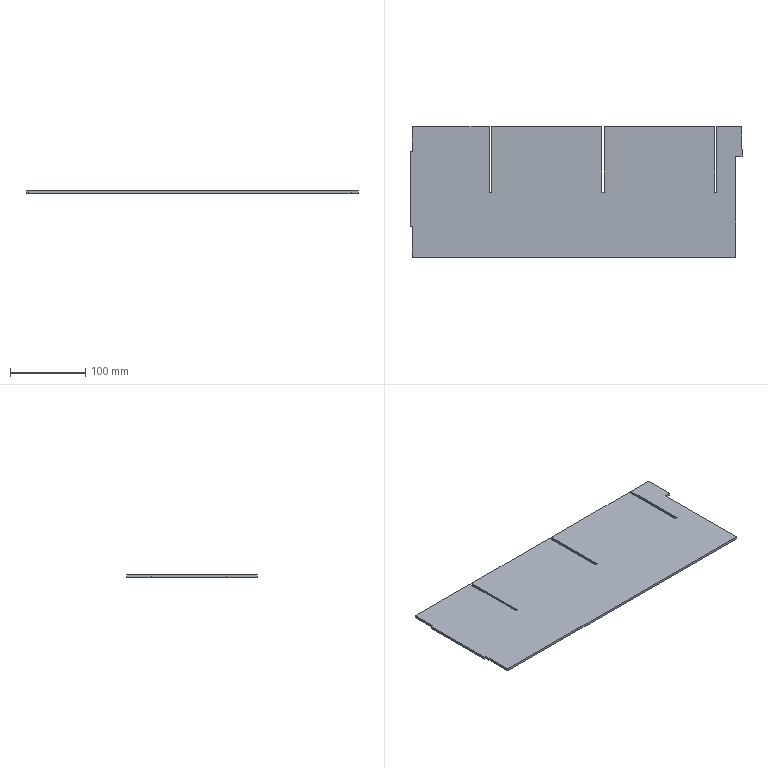Part | SolidWorks | features FlatPattern 1, SMBaseFlange 1, SheetMetal 1 | 1 solid | 24 faces | box 442 x 173.7 x 3.2 mm | volume 238742 mm3 | plane 24
STEP:
#1=CARTESIAN_POINT('',(-658.5,-13.627,0.));
#2=VERTEX_POINT('',#1);
#3=CARTESIAN_POINT('',(-658.5,-46.127,0.));
#4=VERTEX_POINT('',#3);
#5=CARTESIAN_POINT('',(-658.5,-13.627,0.));
#6=DIRECTION('',(0.,-1.,0.));
#7=VECTOR('',#6,1000.);
#8=LINE('',#5,#7);
#9=EDGE_CURVE('',#2,#4,#8,.T.);
#10=ORIENTED_EDGE('',*,*,#9,.T.);
#11=CARTESIAN_POINT('',(-658.5,-46.127,3.2));
#12=VERTEX_POINT('',#11);
#13=CARTESIAN_POINT('',(-658.5,-46.127,3.2));
#14=DIRECTION('',(0.,0.,-1.));
#15=VECTOR('',#14,1000.);
#16=LINE('',#13,#15);
#17=EDGE_CURVE('',#12,#4,#16,.T.);
#18=ORIENTED_EDGE('',*,*,#17,.F.);
#19=CARTESIAN_POINT('',(-658.5,-13.627,3.2));
#20=VERTEX_POINT('',#19);
#21=CARTESIAN_POINT('',(-658.5,-13.627,3.2));
#22=DIRECTION('',(0.,-1.,0.));
#23=VECTOR('',#22,1000.);
#24=LINE('',#21,#23);
#25=EDGE_CURVE('',#20,#12,#24,.T.);
#26=ORIENTED_EDGE('',*,*,#25,.F.);
#27=CARTESIAN_POINT('',(-658.5,-13.627,3.2));
#28=DIRECTION('',(0.,0.,-1.));
#29=VECTOR('',#28,1000.);
#30=LINE('',#27,#29);
#31=EDGE_CURVE('',#20,#2,#30,.T.);
#32=ORIENTED_EDGE('',*,*,#31,.T.);
#33=EDGE_LOOP('',(#10,#18,#26,#32));
#34=FACE_OUTER_BOUND('',#33,.T.);
#35=CARTESIAN_POINT('',(-658.5,-13.627,3.2));
#36=DIRECTION('',(1.,0.,0.));
#37=DIRECTION('',(0.,1.,0.));
#38=AXIS2_PLACEMENT_3D('',#35,#36,#37);
#39=PLANE('',#38);
#40=ADVANCED_FACE('',(#34),#39,.F.);
#41=CARTESIAN_POINT('',(-661.5,-46.127,0.));
#42=VERTEX_POINT('',#41);
#43=CARTESIAN_POINT('',(-658.5,-46.127,0.));
#44=DIRECTION('',(-1.,0.,0.));
#45=VECTOR('',#44,1000.);
#46=LINE('',#43,#45);
#47=EDGE_CURVE('',#4,#42,#46,.T.);
#48=ORIENTED_EDGE('',*,*,#47,.T.);
#49=CARTESIAN_POINT('',(-661.5,-46.127,3.2));
#50=VERTEX_POINT('',#49);
#51=CARTESIAN_POINT('',(-661.5,-46.127,3.2));
#52=DIRECTION('',(0.,0.,-1.));
#53=VECTOR('',#52,1000.);
#54=LINE('',#51,#53);
#55=EDGE_CURVE('',#50,#42,#54,.T.);
#56=ORIENTED_EDGE('',*,*,#55,.F.);
#57=CARTESIAN_POINT('',(-658.5,-46.127,3.2));
#58=DIRECTION('',(-1.,0.,0.));
#59=VECTOR('',#58,1000.);
#60=LINE('',#57,#59);
#61=EDGE_CURVE('',#12,#50,#60,.T.);
#62=ORIENTED_EDGE('',*,*,#61,.F.);
#63=ORIENTED_EDGE('',*,*,#17,.T.);
#64=EDGE_LOOP('',(#48,#56,#62,#63));
#65=FACE_OUTER_BOUND('',#64,.T.);
#66=CARTESIAN_POINT('',(-658.5,-46.127,3.2));
#67=DIRECTION('',(0.,-1.,0.));
#68=DIRECTION('',(1.,0.,0.));
#69=AXIS2_PLACEMENT_3D('',#66,#67,#68);
#70=PLANE('',#69);
#71=ADVANCED_FACE('',(#65),#70,.F.);
#72=CARTESIAN_POINT('',(-661.5,-146.127,0.));
#73=VERTEX_POINT('',#72);
#74=CARTESIAN_POINT('',(-661.5,-46.127,0.));
#75=DIRECTION('',(0.,-1.,0.));
#76=VECTOR('',#75,1000.);
#77=LINE('',#74,#76);
#78=EDGE_CURVE('',#42,#73,#77,.T.);
#79=ORIENTED_EDGE('',*,*,#78,.T.);
#80=CARTESIAN_POINT('',(-661.5,-146.127,3.2));
#81=VERTEX_POINT('',#80);
#82=CARTESIAN_POINT('',(-661.5,-146.127,3.2));
#83=DIRECTION('',(0.,0.,-1.));
#84=VECTOR('',#83,1000.);
#85=LINE('',#82,#84);
#86=EDGE_CURVE('',#81,#73,#85,.T.);
#87=ORIENTED_EDGE('',*,*,#86,.F.);
#88=CARTESIAN_POINT('',(-661.5,-46.127,3.2));
#89=DIRECTION('',(0.,-1.,0.));
#90=VECTOR('',#89,1000.);
#91=LINE('',#88,#90);
#92=EDGE_CURVE('',#50,#81,#91,.T.);
#93=ORIENTED_EDGE('',*,*,#92,.F.);
#94=ORIENTED_EDGE('',*,*,#55,.T.);
#95=EDGE_LOOP('',(#79,#87,#93,#94));
#96=FACE_OUTER_BOUND('',#95,.T.);
#97=CARTESIAN_POINT('',(-661.5,-46.127,3.2));
#98=DIRECTION('',(1.,0.,0.));
#99=DIRECTION('',(0.,1.,0.));
#100=AXIS2_PLACEMENT_3D('',#97,#98,#99);
#101=PLANE('',#100);
#102=ADVANCED_FACE('',(#96),#101,.F.);
#103=CARTESIAN_POINT('',(-658.5,-146.127,0.));
#104=VERTEX_POINT('',#103);
#105=CARTESIAN_POINT('',(-658.5,-146.127,0.));
#106=DIRECTION('',(1.,0.,0.));
#107=VECTOR('',#106,1000.);
#108=LINE('',#105,#107);
#109=EDGE_CURVE('',#73,#104,#108,.T.);
#110=ORIENTED_EDGE('',*,*,#109,.T.);
#111=CARTESIAN_POINT('',(-658.5,-146.127,3.2));
#112=VERTEX_POINT('',#111);
#113=CARTESIAN_POINT('',(-658.5,-146.127,3.2));
#114=DIRECTION('',(0.,0.,-1.));
#115=VECTOR('',#114,1000.);
#116=LINE('',#113,#115);
#117=EDGE_CURVE('',#112,#104,#116,.T.);
#118=ORIENTED_EDGE('',*,*,#117,.F.);
#119=CARTESIAN_POINT('',(-658.5,-146.127,3.2));
#120=DIRECTION('',(1.,0.,0.));
#121=VECTOR('',#120,1000.);
#122=LINE('',#119,#121);
#123=EDGE_CURVE('',#81,#112,#122,.T.);
#124=ORIENTED_EDGE('',*,*,#123,.F.);
#125=ORIENTED_EDGE('',*,*,#86,.T.);
#126=EDGE_LOOP('',(#110,#118,#124,#125));
#127=FACE_OUTER_BOUND('',#126,.T.);
#128=CARTESIAN_POINT('',(-658.5,-146.127,3.2));
#129=DIRECTION('',(0.,1.,0.));
#130=DIRECTION('',(0.,0.,1.));
#131=AXIS2_PLACEMENT_3D('',#128,#129,#130);
#132=PLANE('',#131);
#133=ADVANCED_FACE('',(#127),#132,.F.);
#134=CARTESIAN_POINT('',(-658.5,-187.327,0.));
#135=VERTEX_POINT('',#134);
#136=CARTESIAN_POINT('',(-658.5,-146.127,0.));
#137=DIRECTION('',(0.,-1.,0.));
#138=VECTOR('',#137,1000.);
#139=LINE('',#136,#138);
#140=EDGE_CURVE('',#104,#135,#139,.T.);
#141=ORIENTED_EDGE('',*,*,#140,.T.);
#142=CARTESIAN_POINT('',(-658.5,-187.327,3.2));
#143=VERTEX_POINT('',#142);
#144=CARTESIAN_POINT('',(-658.5,-187.327,3.2));
#145=DIRECTION('',(0.,0.,-1.));
#146=VECTOR('',#145,1000.);
#147=LINE('',#144,#146);
#148=EDGE_CURVE('',#143,#135,#147,.T.);
#149=ORIENTED_EDGE('',*,*,#148,.F.);
#150=CARTESIAN_POINT('',(-658.5,-146.127,3.2));
#151=DIRECTION('',(0.,-1.,0.));
#152=VECTOR('',#151,1000.);
#153=LINE('',#150,#152);
#154=EDGE_CURVE('',#112,#143,#153,.T.);
#155=ORIENTED_EDGE('',*,*,#154,.F.);
#156=ORIENTED_EDGE('',*,*,#117,.T.);
#157=EDGE_LOOP('',(#141,#149,#155,#156));
#158=FACE_OUTER_BOUND('',#157,.T.);
#159=CARTESIAN_POINT('',(-658.5,-146.127,3.2));
#160=DIRECTION('',(1.,0.,0.));
#161=DIRECTION('',(0.,1.,0.));
#162=AXIS2_PLACEMENT_3D('',#159,#160,#161);
#163=PLANE('',#162);
#164=ADVANCED_FACE('',(#158),#163,.F.);
#165=CARTESIAN_POINT('',(-227.8,-187.327,0.));
#166=VERTEX_POINT('',#165);
#167=CARTESIAN_POINT('',(-227.8,-187.327,0.));
#168=DIRECTION('',(1.,0.,0.));
#169=VECTOR('',#168,1000.);
#170=LINE('',#167,#169);
#171=EDGE_CURVE('',#135,#166,#170,.T.);
#172=ORIENTED_EDGE('',*,*,#171,.T.);
#173=CARTESIAN_POINT('',(-227.8,-187.327,3.2));
#174=VERTEX_POINT('',#173);
#175=CARTESIAN_POINT('',(-227.8,-187.327,3.2));
#176=DIRECTION('',(0.,0.,-1.));
#177=VECTOR('',#176,1000.);
#178=LINE('',#175,#177);
#179=EDGE_CURVE('',#174,#166,#178,.T.);
#180=ORIENTED_EDGE('',*,*,#179,.F.);
#181=CARTESIAN_POINT('',(-227.8,-187.327,3.2));
#182=DIRECTION('',(1.,0.,0.));
#183=VECTOR('',#182,1000.);
#184=LINE('',#181,#183);
#185=EDGE_CURVE('',#143,#174,#184,.T.);
#186=ORIENTED_EDGE('',*,*,#185,.F.);
#187=ORIENTED_EDGE('',*,*,#148,.T.);
#188=EDGE_LOOP('',(#172,#180,#186,#187));
#189=FACE_OUTER_BOUND('',#188,.T.);
#190=CARTESIAN_POINT('',(-227.8,-187.327,3.2));
#191=DIRECTION('',(0.,1.,0.));
#192=DIRECTION('',(-1.,0.,0.));
#193=AXIS2_PLACEMENT_3D('',#190,#191,#192);
#194=PLANE('',#193);
#195=ADVANCED_FACE('',(#189),#194,.F.);
#196=CARTESIAN_POINT('',(-227.8,-53.327,0.));
#197=VERTEX_POINT('',#196);
#198=CARTESIAN_POINT('',(-227.8,-53.327,0.));
#199=DIRECTION('',(0.,1.,0.));
#200=VECTOR('',#199,1000.);
#201=LINE('',#198,#200);
#202=EDGE_CURVE('',#166,#197,#201,.T.);
#203=ORIENTED_EDGE('',*,*,#202,.T.);
#204=CARTESIAN_POINT('',(-227.8,-53.327,3.2));
#205=VERTEX_POINT('',#204);
#206=CARTESIAN_POINT('',(-227.8,-53.327,3.2));
#207=DIRECTION('',(0.,0.,-1.));
#208=VECTOR('',#207,1000.);
#209=LINE('',#206,#208);
#210=EDGE_CURVE('',#205,#197,#209,.T.);
#211=ORIENTED_EDGE('',*,*,#210,.F.);
#212=CARTESIAN_POINT('',(-227.8,-53.327,3.2));
#213=DIRECTION('',(0.,1.,0.));
#214=VECTOR('',#213,1000.);
#215=LINE('',#212,#214);
#216=EDGE_CURVE('',#174,#205,#215,.T.);
#217=ORIENTED_EDGE('',*,*,#216,.F.);
#218=ORIENTED_EDGE('',*,*,#179,.T.);
#219=EDGE_LOOP('',(#203,#211,#217,#218));
#220=FACE_OUTER_BOUND('',#219,.T.);
#221=CARTESIAN_POINT('',(-227.8,-53.327,3.2));
#222=DIRECTION('',(-1.,0.,0.));
#223=DIRECTION('',(0.,-1.,0.));
#224=AXIS2_PLACEMENT_3D('',#221,#222,#223);
#225=PLANE('',#224);
#226=ADVANCED_FACE('',(#220),#225,.F.);
#227=CARTESIAN_POINT('',(-219.5,-53.327,0.));
#228=VERTEX_POINT('',#227);
#229=CARTESIAN_POINT('',(-227.8,-53.327,0.));
#230=DIRECTION('',(1.,0.,0.));
#231=VECTOR('',#230,1000.);
#232=LINE('',#229,#231);
#233=EDGE_CURVE('',#197,#228,#232,.T.);
#234=ORIENTED_EDGE('',*,*,#233,.T.);
#235=CARTESIAN_POINT('',(-219.5,-53.327,3.2));
#236=VERTEX_POINT('',#235);
#237=CARTESIAN_POINT('',(-219.5,-53.327,3.2));
#238=DIRECTION('',(0.,0.,-1.));
#239=VECTOR('',#238,1000.);
#240=LINE('',#237,#239);
#241=EDGE_CURVE('',#236,#228,#240,.T.);
#242=ORIENTED_EDGE('',*,*,#241,.F.);
#243=CARTESIAN_POINT('',(-227.8,-53.327,3.2));
#244=DIRECTION('',(1.,0.,0.));
#245=VECTOR('',#244,1000.);
#246=LINE('',#243,#245);
#247=EDGE_CURVE('',#205,#236,#246,.T.);
#248=ORIENTED_EDGE('',*,*,#247,.F.);
#249=ORIENTED_EDGE('',*,*,#210,.T.);
#250=EDGE_LOOP('',(#234,#242,#248,#249));
#251=FACE_OUTER_BOUND('',#250,.T.);
#252=CARTESIAN_POINT('',(-227.8,-53.327,3.2));
#253=DIRECTION('',(0.,1.,0.));
#254=DIRECTION('',(-1.,0.,0.));
#255=AXIS2_PLACEMENT_3D('',#252,#253,#254);
#256=PLANE('',#255);
#257=ADVANCED_FACE('',(#251),#256,.F.);
#258=CARTESIAN_POINT('',(-219.5,-13.627,0.));
#259=VERTEX_POINT('',#258);
#260=CARTESIAN_POINT('',(-219.5,-53.327,0.));
#261=DIRECTION('',(0.,1.,0.));
#262=VECTOR('',#261,1000.);
#263=LINE('',#260,#262);
#264=EDGE_CURVE('',#228,#259,#263,.T.);
#265=ORIENTED_EDGE('',*,*,#264,.T.);
#266=CARTESIAN_POINT('',(-219.5,-13.627,3.2));
#267=VERTEX_POINT('',#266);
#268=CARTESIAN_POINT('',(-219.5,-13.627,3.2));
#269=DIRECTION('',(0.,0.,-1.));
#270=VECTOR('',#269,1000.);
#271=LINE('',#268,#270);
#272=EDGE_CURVE('',#267,#259,#271,.T.);
#273=ORIENTED_EDGE('',*,*,#272,.F.);
#274=CARTESIAN_POINT('',(-219.5,-53.327,3.2));
#275=DIRECTION('',(0.,1.,0.));
#276=VECTOR('',#275,1000.);
#277=LINE('',#274,#276);
#278=EDGE_CURVE('',#236,#267,#277,.T.);
#279=ORIENTED_EDGE('',*,*,#278,.F.);
#280=ORIENTED_EDGE('',*,*,#241,.T.);
#281=EDGE_LOOP('',(#265,#273,#279,#280));
#282=FACE_OUTER_BOUND('',#281,.T.);
#283=CARTESIAN_POINT('',(-219.5,-53.327,3.2));
#284=DIRECTION('',(-1.,0.,0.));
#285=DIRECTION('',(0.,-1.,0.));
#286=AXIS2_PLACEMENT_3D('',#283,#284,#285);
#287=PLANE('',#286);
#288=ADVANCED_FACE('',(#282),#287,.F.);
#289=CARTESIAN_POINT('',(-252.8,-13.627,0.));
#290=VERTEX_POINT('',#289);
#291=CARTESIAN_POINT('',(-219.5,-13.627,0.));
#292=DIRECTION('',(-1.,0.,0.));
#293=VECTOR('',#292,1000.);
#294=LINE('',#291,#293);
#295=EDGE_CURVE('',#259,#290,#294,.T.);
#296=ORIENTED_EDGE('',*,*,#295,.T.);
#297=CARTESIAN_POINT('',(-252.8,-13.627,3.2));
#298=VERTEX_POINT('',#297);
#299=CARTESIAN_POINT('',(-252.8,-13.627,3.2));
#300=DIRECTION('',(0.,0.,-1.));
#301=VECTOR('',#300,1000.);
#302=LINE('',#299,#301);
#303=EDGE_CURVE('',#298,#290,#302,.T.);
#304=ORIENTED_EDGE('',*,*,#303,.F.);
#305=CARTESIAN_POINT('',(-219.5,-13.627,3.2));
#306=DIRECTION('',(-1.,0.,0.));
#307=VECTOR('',#306,1000.);
#308=LINE('',#305,#307);
#309=EDGE_CURVE('',#267,#298,#308,.T.);
#310=ORIENTED_EDGE('',*,*,#309,.F.);
#311=ORIENTED_EDGE('',*,*,#272,.T.);
#312=EDGE_LOOP('',(#296,#304,#310,#311));
#313=FACE_OUTER_BOUND('',#312,.T.);
#314=CARTESIAN_POINT('',(-219.5,-13.627,3.2));
#315=DIRECTION('',(0.,-1.,0.));
#316=DIRECTION('',(1.,0.,0.));
#317=AXIS2_PLACEMENT_3D('',#314,#315,#316);
#318=PLANE('',#317);
#319=ADVANCED_FACE('',(#313),#318,.F.);
#320=CARTESIAN_POINT('',(-252.8,-100.627,0.));
#321=VERTEX_POINT('',#320);
#322=CARTESIAN_POINT('',(-252.8,-13.627,0.));
#323=DIRECTION('',(0.,-1.,0.));
#324=VECTOR('',#323,1000.);
#325=LINE('',#322,#324);
#326=EDGE_CURVE('',#290,#321,#325,.T.);
#327=ORIENTED_EDGE('',*,*,#326,.T.);
#328=CARTESIAN_POINT('',(-252.8,-100.627,3.2));
#329=VERTEX_POINT('',#328);
#330=CARTESIAN_POINT('',(-252.8,-100.627,3.2));
#331=DIRECTION('',(0.,0.,-1.));
#332=VECTOR('',#331,1000.);
#333=LINE('',#330,#332);
#334=EDGE_CURVE('',#329,#321,#333,.T.);
#335=ORIENTED_EDGE('',*,*,#334,.F.);
#336=CARTESIAN_POINT('',(-252.8,-13.627,3.2));
#337=DIRECTION('',(0.,-1.,0.));
#338=VECTOR('',#337,1000.);
#339=LINE('',#336,#338);
#340=EDGE_CURVE('',#298,#329,#339,.T.);
#341=ORIENTED_EDGE('',*,*,#340,.F.);
#342=ORIENTED_EDGE('',*,*,#303,.T.);
#343=EDGE_LOOP('',(#327,#335,#341,#342));
#344=FACE_OUTER_BOUND('',#343,.T.);
#345=CARTESIAN_POINT('',(-252.8,-13.627,3.2));
#346=DIRECTION('',(1.,0.,0.));
#347=DIRECTION('',(0.,0.,-1.));
#348=AXIS2_PLACEMENT_3D('',#345,#346,#347);
#349=PLANE('',#348);
#350=ADVANCED_FACE('',(#344),#349,.F.);
#351=CARTESIAN_POINT('',(-256.,-100.627,0.));
#352=VERTEX_POINT('',#351);
#353=CARTESIAN_POINT('',(-252.8,-100.627,0.));
#354=DIRECTION('',(-1.,0.,0.));
#355=VECTOR('',#354,1000.);
#356=LINE('',#353,#355);
#357=EDGE_CURVE('',#321,#352,#356,.T.);
#358=ORIENTED_EDGE('',*,*,#357,.T.);
#359=CARTESIAN_POINT('',(-256.,-100.627,3.2));
#360=VERTEX_POINT('',#359);
#361=CARTESIAN_POINT('',(-256.,-100.627,3.2));
#362=DIRECTION('',(0.,0.,-1.));
#363=VECTOR('',#362,1000.);
#364=LINE('',#361,#363);
#365=EDGE_CURVE('',#360,#352,#364,.T.);
#366=ORIENTED_EDGE('',*,*,#365,.F.);
#367=CARTESIAN_POINT('',(-252.8,-100.627,3.2));
#368=DIRECTION('',(-1.,0.,0.));
#369=VECTOR('',#368,1000.);
#370=LINE('',#367,#369);
#371=EDGE_CURVE('',#329,#360,#370,.T.);
#372=ORIENTED_EDGE('',*,*,#371,.F.);
#373=ORIENTED_EDGE('',*,*,#334,.T.);
#374=EDGE_LOOP('',(#358,#366,#372,#373));
#375=FACE_OUTER_BOUND('',#374,.T.);
#376=CARTESIAN_POINT('',(-252.8,-100.627,3.2));
#377=DIRECTION('',(0.,-1.,0.));
#378=DIRECTION('',(0.,0.,-1.));
#379=AXIS2_PLACEMENT_3D('',#376,#377,#378);
#380=PLANE('',#379);
#381=ADVANCED_FACE('',(#375),#380,.F.);
#382=CARTESIAN_POINT('',(-256.,-13.627,0.));
#383=VERTEX_POINT('',#382);
#384=CARTESIAN_POINT('',(-256.,-100.627,0.));
#385=DIRECTION('',(0.,1.,0.));
#386=VECTOR('',#385,1000.);
#387=LINE('',#384,#386);
#388=EDGE_CURVE('',#352,#383,#387,.T.);
#389=ORIENTED_EDGE('',*,*,#388,.T.);
#390=CARTESIAN_POINT('',(-256.,-13.627,3.2));
#391=VERTEX_POINT('',#390);
#392=CARTESIAN_POINT('',(-256.,-13.627,3.2));
#393=DIRECTION('',(0.,0.,-1.));
#394=VECTOR('',#393,1000.);
#395=LINE('',#392,#394);
#396=EDGE_CURVE('',#391,#383,#395,.T.);
#397=ORIENTED_EDGE('',*,*,#396,.F.);
#398=CARTESIAN_POINT('',(-256.,-100.627,3.2));
#399=DIRECTION('',(0.,1.,0.));
#400=VECTOR('',#399,1000.);
#401=LINE('',#398,#400);
#402=EDGE_CURVE('',#360,#391,#401,.T.);
#403=ORIENTED_EDGE('',*,*,#402,.F.);
#404=ORIENTED_EDGE('',*,*,#365,.T.);
#405=EDGE_LOOP('',(#389,#397,#403,#404));
#406=FACE_OUTER_BOUND('',#405,.T.);
#407=CARTESIAN_POINT('',(-256.,-100.627,3.2));
#408=DIRECTION('',(-1.,0.,0.));
#409=DIRECTION('',(0.,0.,1.));
#410=AXIS2_PLACEMENT_3D('',#407,#408,#409);
#411=PLANE('',#410);
#412=ADVANCED_FACE('',(#406),#411,.F.);
#413=CARTESIAN_POINT('',(-402.8,-13.627,0.));
#414=VERTEX_POINT('',#413);
#415=CARTESIAN_POINT('',(-256.,-13.627,0.));
#416=DIRECTION('',(-1.,0.,0.));
#417=VECTOR('',#416,1000.);
#418=LINE('',#415,#417);
#419=EDGE_CURVE('',#383,#414,#418,.T.);
#420=ORIENTED_EDGE('',*,*,#419,.T.);
#421=CARTESIAN_POINT('',(-402.8,-13.627,3.2));
#422=VERTEX_POINT('',#421);
#423=CARTESIAN_POINT('',(-402.8,-13.627,3.2));
#424=DIRECTION('',(0.,0.,-1.));
#425=VECTOR('',#424,1000.);
#426=LINE('',#423,#425);
#427=EDGE_CURVE('',#422,#414,#426,.T.);
#428=ORIENTED_EDGE('',*,*,#427,.F.);
#429=CARTESIAN_POINT('',(-256.,-13.627,3.2));
#430=DIRECTION('',(-1.,0.,0.));
#431=VECTOR('',#430,1000.);
#432=LINE('',#429,#431);
#433=EDGE_CURVE('',#391,#422,#432,.T.);
#434=ORIENTED_EDGE('',*,*,#433,.F.);
#435=ORIENTED_EDGE('',*,*,#396,.T.);
#436=EDGE_LOOP('',(#420,#428,#434,#435));
#437=FACE_OUTER_BOUND('',#436,.T.);
#438=CARTESIAN_POINT('',(-256.,-13.627,3.2));
#439=DIRECTION('',(0.,-1.,0.));
#440=DIRECTION('',(1.,0.,0.));
#441=AXIS2_PLACEMENT_3D('',#438,#439,#440);
#442=PLANE('',#441);
#443=ADVANCED_FACE('',(#437),#442,.F.);
#444=CARTESIAN_POINT('',(-402.8,-100.627,0.));
#445=VERTEX_POINT('',#444);
#446=CARTESIAN_POINT('',(-402.8,-13.627,0.));
#447=DIRECTION('',(0.,-1.,0.));
#448=VECTOR('',#447,1000.);
#449=LINE('',#446,#448);
#450=EDGE_CURVE('',#414,#445,#449,.T.);
#451=ORIENTED_EDGE('',*,*,#450,.T.);
#452=CARTESIAN_POINT('',(-402.8,-100.627,3.2));
#453=VERTEX_POINT('',#452);
#454=CARTESIAN_POINT('',(-402.8,-100.627,3.2));
#455=DIRECTION('',(0.,0.,-1.));
#456=VECTOR('',#455,1000.);
#457=LINE('',#454,#456);
#458=EDGE_CURVE('',#453,#445,#457,.T.);
#459=ORIENTED_EDGE('',*,*,#458,.F.);
#460=CARTESIAN_POINT('',(-402.8,-13.627,3.2));
#461=DIRECTION('',(0.,-1.,0.));
#462=VECTOR('',#461,1000.);
#463=LINE('',#460,#462);
#464=EDGE_CURVE('',#422,#453,#463,.T.);
#465=ORIENTED_EDGE('',*,*,#464,.F.);
#466=ORIENTED_EDGE('',*,*,#427,.T.);
#467=EDGE_LOOP('',(#451,#459,#465,#466));
#468=FACE_OUTER_BOUND('',#467,.T.);
#469=CARTESIAN_POINT('',(-402.8,-13.627,3.2));
#470=DIRECTION('',(1.,0.,0.));
#471=DIRECTION('',(0.,1.,0.));
#472=AXIS2_PLACEMENT_3D('',#469,#470,#471);
#473=PLANE('',#472);
#474=ADVANCED_FACE('',(#468),#473,.F.);
#475=CARTESIAN_POINT('',(-406.,-100.627,0.));
#476=VERTEX_POINT('',#475);
#477=CARTESIAN_POINT('',(-402.8,-100.627,0.));
#478=DIRECTION('',(-1.,0.,0.));
#479=VECTOR('',#478,1000.);
#480=LINE('',#477,#479);
#481=EDGE_CURVE('',#445,#476,#480,.T.);
#482=ORIENTED_EDGE('',*,*,#481,.T.);
#483=CARTESIAN_POINT('',(-406.,-100.627,3.2));
#484=VERTEX_POINT('',#483);
#485=CARTESIAN_POINT('',(-406.,-100.627,3.2));
#486=DIRECTION('',(0.,0.,-1.));
#487=VECTOR('',#486,1000.);
#488=LINE('',#485,#487);
#489=EDGE_CURVE('',#484,#476,#488,.T.);
#490=ORIENTED_EDGE('',*,*,#489,.F.);
#491=CARTESIAN_POINT('',(-402.8,-100.627,3.2));
#492=DIRECTION('',(-1.,0.,0.));
#493=VECTOR('',#492,1000.);
#494=LINE('',#491,#493);
#495=EDGE_CURVE('',#453,#484,#494,.T.);
#496=ORIENTED_EDGE('',*,*,#495,.F.);
#497=ORIENTED_EDGE('',*,*,#458,.T.);
#498=EDGE_LOOP('',(#482,#490,#496,#497));
#499=FACE_OUTER_BOUND('',#498,.T.);
#500=CARTESIAN_POINT('',(-402.8,-100.627,3.2));
#501=DIRECTION('',(0.,-1.,0.));
#502=DIRECTION('',(0.,0.,-1.));
#503=AXIS2_PLACEMENT_3D('',#500,#501,#502);
#504=PLANE('',#503);
#505=ADVANCED_FACE('',(#499),#504,.F.);
#506=CARTESIAN_POINT('',(-406.,-13.627,0.));
#507=VERTEX_POINT('',#506);
#508=CARTESIAN_POINT('',(-406.,-100.627,0.));
#509=DIRECTION('',(0.,1.,0.));
#510=VECTOR('',#509,1000.);
#511=LINE('',#508,#510);
#512=EDGE_CURVE('',#476,#507,#511,.T.);
#513=ORIENTED_EDGE('',*,*,#512,.T.);
#514=CARTESIAN_POINT('',(-406.,-13.627,3.2));
#515=VERTEX_POINT('',#514);
#516=CARTESIAN_POINT('',(-406.,-13.627,3.2));
#517=DIRECTION('',(0.,0.,-1.));
#518=VECTOR('',#517,1000.);
#519=LINE('',#516,#518);
#520=EDGE_CURVE('',#515,#507,#519,.T.);
#521=ORIENTED_EDGE('',*,*,#520,.F.);
#522=CARTESIAN_POINT('',(-406.,-100.627,3.2));
#523=DIRECTION('',(0.,1.,0.));
#524=VECTOR('',#523,1000.);
#525=LINE('',#522,#524);
#526=EDGE_CURVE('',#484,#515,#525,.T.);
#527=ORIENTED_EDGE('',*,*,#526,.F.);
#528=ORIENTED_EDGE('',*,*,#489,.T.);
#529=EDGE_LOOP('',(#513,#521,#527,#528));
#530=FACE_OUTER_BOUND('',#529,.T.);
#531=CARTESIAN_POINT('',(-406.,-100.627,3.2));
#532=DIRECTION('',(-1.,0.,0.));
#533=DIRECTION('',(0.,-1.,0.));
#534=AXIS2_PLACEMENT_3D('',#531,#532,#533);
#535=PLANE('',#534);
#536=ADVANCED_FACE('',(#530),#535,.F.);
#537=CARTESIAN_POINT('',(-552.8,-13.627,0.));
#538=VERTEX_POINT('',#537);
#539=CARTESIAN_POINT('',(-406.,-13.627,0.));
#540=DIRECTION('',(-1.,0.,0.));
#541=VECTOR('',#540,1000.);
#542=LINE('',#539,#541);
#543=EDGE_CURVE('',#507,#538,#542,.T.);
#544=ORIENTED_EDGE('',*,*,#543,.T.);
#545=CARTESIAN_POINT('',(-552.8,-13.627,3.2));
#546=VERTEX_POINT('',#545);
#547=CARTESIAN_POINT('',(-552.8,-13.627,3.2));
#548=DIRECTION('',(0.,0.,-1.));
#549=VECTOR('',#548,1000.);
#550=LINE('',#547,#549);
#551=EDGE_CURVE('',#546,#538,#550,.T.);
#552=ORIENTED_EDGE('',*,*,#551,.F.);
#553=CARTESIAN_POINT('',(-406.,-13.627,3.2));
#554=DIRECTION('',(-1.,0.,0.));
#555=VECTOR('',#554,1000.);
#556=LINE('',#553,#555);
#557=EDGE_CURVE('',#515,#546,#556,.T.);
#558=ORIENTED_EDGE('',*,*,#557,.F.);
#559=ORIENTED_EDGE('',*,*,#520,.T.);
#560=EDGE_LOOP('',(#544,#552,#558,#559));
#561=FACE_OUTER_BOUND('',#560,.T.);
#562=CARTESIAN_POINT('',(-406.,-13.627,3.2));
#563=DIRECTION('',(0.,-1.,0.));
#564=DIRECTION('',(1.,0.,0.));
#565=AXIS2_PLACEMENT_3D('',#562,#563,#564);
#566=PLANE('',#565);
#567=ADVANCED_FACE('',(#561),#566,.F.);
#568=CARTESIAN_POINT('',(-552.8,-100.627,0.));
#569=VERTEX_POINT('',#568);
#570=CARTESIAN_POINT('',(-552.8,-13.627,0.));
#571=DIRECTION('',(0.,-1.,0.));
#572=VECTOR('',#571,1000.);
#573=LINE('',#570,#572);
#574=EDGE_CURVE('',#538,#569,#573,.T.);
#575=ORIENTED_EDGE('',*,*,#574,.T.);
#576=CARTESIAN_POINT('',(-552.8,-100.627,3.2));
#577=VERTEX_POINT('',#576);
#578=CARTESIAN_POINT('',(-552.8,-100.627,3.2));
#579=DIRECTION('',(0.,0.,-1.));
#580=VECTOR('',#579,1000.);
#581=LINE('',#578,#580);
#582=EDGE_CURVE('',#577,#569,#581,.T.);
#583=ORIENTED_EDGE('',*,*,#582,.F.);
#584=CARTESIAN_POINT('',(-552.8,-13.627,3.2));
#585=DIRECTION('',(0.,-1.,0.));
#586=VECTOR('',#585,1000.);
#587=LINE('',#584,#586);
#588=EDGE_CURVE('',#546,#577,#587,.T.);
#589=ORIENTED_EDGE('',*,*,#588,.F.);
#590=ORIENTED_EDGE('',*,*,#551,.T.);
#591=EDGE_LOOP('',(#575,#583,#589,#590));
#592=FACE_OUTER_BOUND('',#591,.T.);
#593=CARTESIAN_POINT('',(-552.8,-13.627,3.2));
#594=DIRECTION('',(1.,0.,0.));
#595=DIRECTION('',(0.,1.,0.));
#596=AXIS2_PLACEMENT_3D('',#593,#594,#595);
#597=PLANE('',#596);
#598=ADVANCED_FACE('',(#592),#597,.F.);
#599=CARTESIAN_POINT('',(-556.,-100.627,0.));
#600=VERTEX_POINT('',#599);
#601=CARTESIAN_POINT('',(-552.8,-100.627,0.));
#602=DIRECTION('',(-1.,0.,0.));
#603=VECTOR('',#602,1000.);
#604=LINE('',#601,#603);
#605=EDGE_CURVE('',#569,#600,#604,.T.);
#606=ORIENTED_EDGE('',*,*,#605,.T.);
#607=CARTESIAN_POINT('',(-556.,-100.627,3.2));
#608=VERTEX_POINT('',#607);
#609=CARTESIAN_POINT('',(-556.,-100.627,3.2));
#610=DIRECTION('',(0.,0.,-1.));
#611=VECTOR('',#610,1000.);
#612=LINE('',#609,#611);
#613=EDGE_CURVE('',#608,#600,#612,.T.);
#614=ORIENTED_EDGE('',*,*,#613,.F.);
#615=CARTESIAN_POINT('',(-552.8,-100.627,3.2));
#616=DIRECTION('',(-1.,0.,0.));
#617=VECTOR('',#616,1000.);
#618=LINE('',#615,#617);
#619=EDGE_CURVE('',#577,#608,#618,.T.);
#620=ORIENTED_EDGE('',*,*,#619,.F.);
#621=ORIENTED_EDGE('',*,*,#582,.T.);
#622=EDGE_LOOP('',(#606,#614,#620,#621));
#623=FACE_OUTER_BOUND('',#622,.T.);
#624=CARTESIAN_POINT('',(-552.8,-100.627,3.2));
#625=DIRECTION('',(0.,-1.,0.));
#626=DIRECTION('',(0.,0.,-1.));
#627=AXIS2_PLACEMENT_3D('',#624,#625,#626);
#628=PLANE('',#627);
#629=ADVANCED_FACE('',(#623),#628,.F.);
#630=CARTESIAN_POINT('',(-556.,-13.627,0.));
#631=VERTEX_POINT('',#630);
#632=CARTESIAN_POINT('',(-556.,-100.627,0.));
#633=DIRECTION('',(0.,1.,0.));
#634=VECTOR('',#633,1000.);
#635=LINE('',#632,#634);
#636=EDGE_CURVE('',#600,#631,#635,.T.);
#637=ORIENTED_EDGE('',*,*,#636,.T.);
#638=CARTESIAN_POINT('',(-556.,-13.627,3.2));
#639=VERTEX_POINT('',#638);
#640=CARTESIAN_POINT('',(-556.,-13.627,3.2));
#641=DIRECTION('',(0.,0.,-1.));
#642=VECTOR('',#641,1000.);
#643=LINE('',#640,#642);
#644=EDGE_CURVE('',#639,#631,#643,.T.);
#645=ORIENTED_EDGE('',*,*,#644,.F.);
#646=CARTESIAN_POINT('',(-556.,-100.627,3.2));
#647=DIRECTION('',(0.,1.,0.));
#648=VECTOR('',#647,1000.);
#649=LINE('',#646,#648);
#650=EDGE_CURVE('',#608,#639,#649,.T.);
#651=ORIENTED_EDGE('',*,*,#650,.F.);
#652=ORIENTED_EDGE('',*,*,#613,.T.);
#653=EDGE_LOOP('',(#637,#645,#651,#652));
#654=FACE_OUTER_BOUND('',#653,.T.);
#655=CARTESIAN_POINT('',(-556.,-100.627,3.2));
#656=DIRECTION('',(-1.,0.,0.));
#657=DIRECTION('',(0.,-1.,0.));
#658=AXIS2_PLACEMENT_3D('',#655,#656,#657);
#659=PLANE('',#658);
#660=ADVANCED_FACE('',(#654),#659,.F.);
#661=CARTESIAN_POINT('',(-556.,-13.627,0.));
#662=DIRECTION('',(-1.,0.,0.));
#663=VECTOR('',#662,1000.);
#664=LINE('',#661,#663);
#665=EDGE_CURVE('',#631,#2,#664,.T.);
#666=ORIENTED_EDGE('',*,*,#665,.T.);
#667=ORIENTED_EDGE('',*,*,#31,.F.);
#668=CARTESIAN_POINT('',(-556.,-13.627,3.2));
#669=DIRECTION('',(-1.,0.,0.));
#670=VECTOR('',#669,1000.);
#671=LINE('',#668,#670);
#672=EDGE_CURVE('',#639,#20,#671,.T.);
#673=ORIENTED_EDGE('',*,*,#672,.F.);
#674=ORIENTED_EDGE('',*,*,#644,.T.);
#675=EDGE_LOOP('',(#666,#667,#673,#674));
#676=FACE_OUTER_BOUND('',#675,.T.);
#677=CARTESIAN_POINT('',(-556.,-13.627,3.2));
#678=DIRECTION('',(0.,-1.,0.));
#679=DIRECTION('',(1.,0.,0.));
#680=AXIS2_PLACEMENT_3D('',#677,#678,#679);
#681=PLANE('',#680);
#682=ADVANCED_FACE('',(#676),#681,.F.);
#683=ORIENTED_EDGE('',*,*,#25,.T.);
#684=ORIENTED_EDGE('',*,*,#61,.T.);
#685=ORIENTED_EDGE('',*,*,#92,.T.);
#686=ORIENTED_EDGE('',*,*,#123,.T.);
#687=ORIENTED_EDGE('',*,*,#154,.T.);
#688=ORIENTED_EDGE('',*,*,#185,.T.);
#689=ORIENTED_EDGE('',*,*,#216,.T.);
#690=ORIENTED_EDGE('',*,*,#247,.T.);
#691=ORIENTED_EDGE('',*,*,#278,.T.);
#692=ORIENTED_EDGE('',*,*,#309,.T.);
#693=ORIENTED_EDGE('',*,*,#340,.T.);
#694=ORIENTED_EDGE('',*,*,#371,.T.);
#695=ORIENTED_EDGE('',*,*,#402,.T.);
#696=ORIENTED_EDGE('',*,*,#433,.T.);
#697=ORIENTED_EDGE('',*,*,#464,.T.);
#698=ORIENTED_EDGE('',*,*,#495,.T.);
#699=ORIENTED_EDGE('',*,*,#526,.T.);
#700=ORIENTED_EDGE('',*,*,#557,.T.);
#701=ORIENTED_EDGE('',*,*,#588,.T.);
#702=ORIENTED_EDGE('',*,*,#619,.T.);
#703=ORIENTED_EDGE('',*,*,#650,.T.);
#704=ORIENTED_EDGE('',*,*,#672,.T.);
#705=EDGE_LOOP('',(#683,#684,#685,#686,#687,#688,#689,#690,#691,#692,#693,#694,#695,#696,#697,#698,#699,#700,#701,#702,#703,#704));
#706=FACE_OUTER_BOUND('',#705,.T.);
#707=CARTESIAN_POINT('',(0.,0.,3.2));
#708=DIRECTION('',(0.,0.,-1.));
#709=DIRECTION('',(-1.,0.,0.));
#710=AXIS2_PLACEMENT_3D('',#707,#708,#709);
#711=PLANE('',#710);
#712=ADVANCED_FACE('',(#706),#711,.F.);
#713=ORIENTED_EDGE('',*,*,#9,.F.);
#714=ORIENTED_EDGE('',*,*,#665,.F.);
#715=ORIENTED_EDGE('',*,*,#636,.F.);
#716=ORIENTED_EDGE('',*,*,#605,.F.);
#717=ORIENTED_EDGE('',*,*,#574,.F.);
#718=ORIENTED_EDGE('',*,*,#543,.F.);
#719=ORIENTED_EDGE('',*,*,#512,.F.);
#720=ORIENTED_EDGE('',*,*,#481,.F.);
#721=ORIENTED_EDGE('',*,*,#450,.F.);
#722=ORIENTED_EDGE('',*,*,#419,.F.);
#723=ORIENTED_EDGE('',*,*,#388,.F.);
#724=ORIENTED_EDGE('',*,*,#357,.F.);
#725=ORIENTED_EDGE('',*,*,#326,.F.);
#726=ORIENTED_EDGE('',*,*,#295,.F.);
#727=ORIENTED_EDGE('',*,*,#264,.F.);
#728=ORIENTED_EDGE('',*,*,#233,.F.);
#729=ORIENTED_EDGE('',*,*,#202,.F.);
#730=ORIENTED_EDGE('',*,*,#171,.F.);
#731=ORIENTED_EDGE('',*,*,#140,.F.);
#732=ORIENTED_EDGE('',*,*,#109,.F.);
#733=ORIENTED_EDGE('',*,*,#78,.F.);
#734=ORIENTED_EDGE('',*,*,#47,.F.);
#735=EDGE_LOOP('',(#713,#714,#715,#716,#717,#718,#719,#720,#721,#722,#723,#724,#725,#726,#727,#728,#729,#730,#731,#732,#733,#734));
#736=FACE_OUTER_BOUND('',#735,.T.);
#737=CARTESIAN_POINT('',(0.,0.,0.));
#738=DIRECTION('',(0.,0.,-1.));
#739=DIRECTION('',(-1.,0.,0.));
#740=AXIS2_PLACEMENT_3D('',#737,#738,#739);
#741=PLANE('',#740);
#742=ADVANCED_FACE('',(#736),#741,.T.);
#743=CLOSED_SHELL('',(#40,#71,#102,#133,#164,#195,#226,#257,#288,#319,#350,#381,#412,#443,#474,#505,#536,#567,#598,#629,#660,#682,#712,#742));
#744=MANIFOLD_SOLID_BREP('',#743);
#745=CARTESIAN_POINT('',(0.,0.,0.));
#746=DIRECTION('',(0.,0.,1.));
#747=DIRECTION('',(1.,0.,0.));
#748=AXIS2_PLACEMENT_3D('',#745,#746,#747);
#749=(LENGTH_UNIT()NAMED_UNIT(*)SI_UNIT(.MILLI.,.METRE.));
#750=UNCERTAINTY_MEASURE_WITH_UNIT(LENGTH_MEASURE(0.00001),#749,'','');
#751=(NAMED_UNIT(*)PLANE_ANGLE_UNIT()SI_UNIT($,.RADIAN.));
#752=(NAMED_UNIT(*)SI_UNIT($,.STERADIAN.)SOLID_ANGLE_UNIT());
#753=(GEOMETRIC_REPRESENTATION_CONTEXT(3)GLOBAL_UNCERTAINTY_ASSIGNED_CONTEXT((#750))GLOBAL_UNIT_ASSIGNED_CONTEXT((#749,#751,#752))REPRESENTATION_CONTEXT('',''));
#754=ADVANCED_BREP_SHAPE_REPRESENTATION('',(#744,#748),#753);